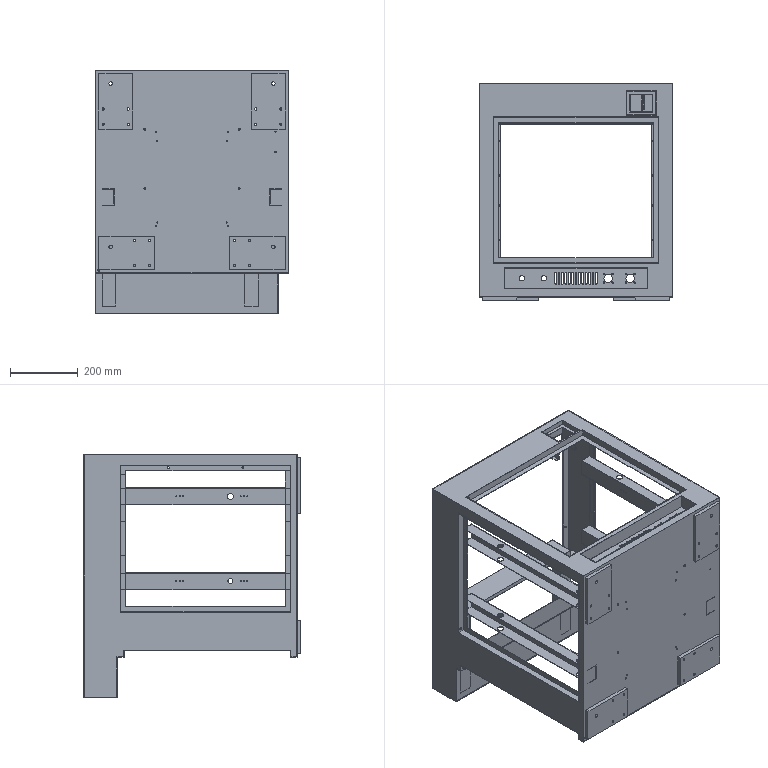Part | SolidWorks | features ICE 78, HoleWzd 16, 3DProfileFeature 7, Fillet 5, Cut 3, LPattern 2, MoveFace 2, Chamfer 1, Extrusion 1, MirrorPattern 1 | 1 solid | 619 faces | box 570 x 640 x 720 mm | volume 3281506 mm3 | plane 314 | cylinder 305 | commonest cylinder face diameters 5 x78 3.3 x72 18 x36 6.8 x32 4 x16 6.5 x14